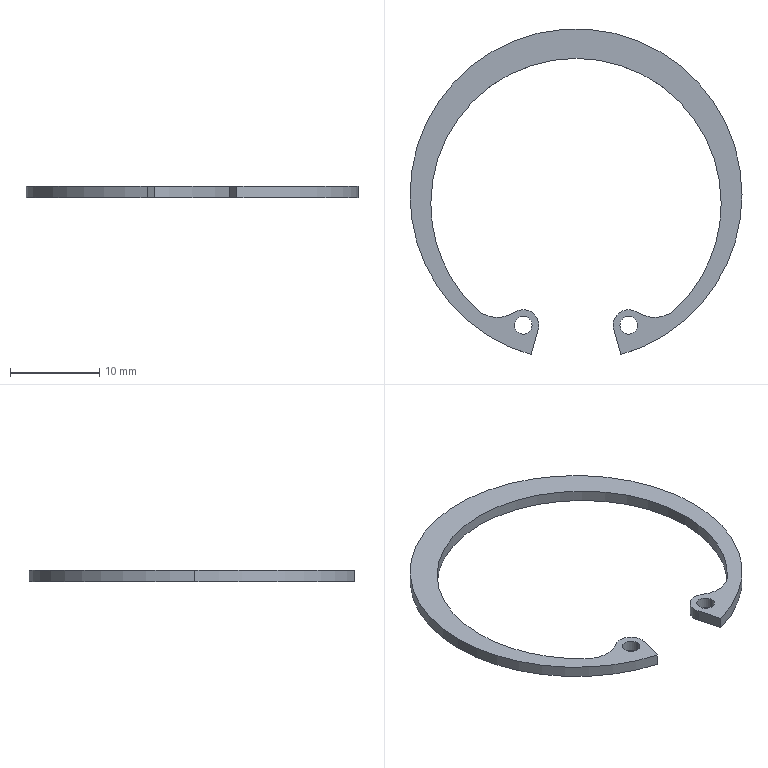Part | STEP file | basic internal retaining ring_wti.25698_Truarc N5000-137 - S1.375 | 1 solid | 19 faces | box 37.109 x 36.419 x 1.27 mm | volume 328.567 mm3 | cylinder 15 | plane 4 | commonest cylinder face diameters 1.981 x4 3.48 x3 32.455 x3 37.109 x3 6.96 x2
STEP:
#1=CARTESIAN_POINT('',(-6.888,-14.575,-1.27));
#2=VERTEX_POINT('',#1);
#3=CARTESIAN_POINT('',(-4.907,-14.575,-1.27));
#4=VERTEX_POINT('',#3);
#5=CARTESIAN_POINT('',(-5.898,-14.575,-1.27));
#6=DIRECTION('',(0.,0.,1.));
#7=DIRECTION('',(1.,0.,0.));
#8=AXIS2_PLACEMENT_3D('',#5,#6,#7);
#9=CIRCLE('',#8,0.9906);
#10=EDGE_CURVE('',#2,#4,#9,.T.);
#11=ORIENTED_EDGE('',*,*,#10,.F.);
#12=CARTESIAN_POINT('',(-6.888,-14.575,0.));
#13=VERTEX_POINT('',#12);
#14=CARTESIAN_POINT('',(-6.888,-14.575,-1.27));
#15=DIRECTION('',(0.,0.,1.));
#16=VECTOR('',#15,1000.);
#17=LINE('',#14,#16);
#18=EDGE_CURVE('',#2,#13,#17,.T.);
#19=ORIENTED_EDGE('',*,*,#18,.T.);
#20=CARTESIAN_POINT('',(-4.907,-14.575,0.));
#21=VERTEX_POINT('',#20);
#22=CARTESIAN_POINT('',(-5.898,-14.575,0.));
#23=DIRECTION('',(0.,0.,1.));
#24=DIRECTION('',(1.,0.,0.));
#25=AXIS2_PLACEMENT_3D('',#22,#23,#24);
#26=CIRCLE('',#25,0.9906);
#27=EDGE_CURVE('',#13,#21,#26,.T.);
#28=ORIENTED_EDGE('',*,*,#27,.T.);
#29=CARTESIAN_POINT('',(-4.907,-14.575,-1.27));
#30=DIRECTION('',(0.,0.,1.));
#31=VECTOR('',#30,1000.);
#32=LINE('',#29,#31);
#33=EDGE_CURVE('',#4,#21,#32,.T.);
#34=ORIENTED_EDGE('',*,*,#33,.F.);
#35=EDGE_LOOP('',(#11,#19,#28,#34));
#36=FACE_OUTER_BOUND('',#35,.T.);
#37=CARTESIAN_POINT('',(-5.898,-14.575,-1.27));
#38=DIRECTION('',(0.,0.,1.));
#39=DIRECTION('',(1.,0.,0.));
#40=AXIS2_PLACEMENT_3D('',#37,#38,#39);
#41=CYLINDRICAL_SURFACE('',#40,0.9906);
#42=ADVANCED_FACE('',(#36),#41,.F.);
#43=CARTESIAN_POINT('',(4.907,-14.575,-1.27));
#44=VERTEX_POINT('',#43);
#45=CARTESIAN_POINT('',(6.888,-14.575,-1.27));
#46=VERTEX_POINT('',#45);
#47=CARTESIAN_POINT('',(5.898,-14.575,-1.27));
#48=DIRECTION('',(0.,0.,1.));
#49=DIRECTION('',(1.,0.,0.));
#50=AXIS2_PLACEMENT_3D('',#47,#48,#49);
#51=CIRCLE('',#50,0.9906);
#52=EDGE_CURVE('',#44,#46,#51,.T.);
#53=ORIENTED_EDGE('',*,*,#52,.F.);
#54=CARTESIAN_POINT('',(4.907,-14.575,0.));
#55=VERTEX_POINT('',#54);
#56=CARTESIAN_POINT('',(4.907,-14.575,-1.27));
#57=DIRECTION('',(0.,0.,1.));
#58=VECTOR('',#57,1000.);
#59=LINE('',#56,#58);
#60=EDGE_CURVE('',#44,#55,#59,.T.);
#61=ORIENTED_EDGE('',*,*,#60,.T.);
#62=CARTESIAN_POINT('',(6.888,-14.575,0.));
#63=VERTEX_POINT('',#62);
#64=CARTESIAN_POINT('',(5.898,-14.575,0.));
#65=DIRECTION('',(0.,0.,1.));
#66=DIRECTION('',(1.,0.,0.));
#67=AXIS2_PLACEMENT_3D('',#64,#65,#66);
#68=CIRCLE('',#67,0.9906);
#69=EDGE_CURVE('',#55,#63,#68,.T.);
#70=ORIENTED_EDGE('',*,*,#69,.T.);
#71=CARTESIAN_POINT('',(6.888,-14.575,-1.27));
#72=DIRECTION('',(0.,0.,1.));
#73=VECTOR('',#72,1000.);
#74=LINE('',#71,#73);
#75=EDGE_CURVE('',#46,#63,#74,.T.);
#76=ORIENTED_EDGE('',*,*,#75,.F.);
#77=EDGE_LOOP('',(#53,#61,#70,#76));
#78=FACE_OUTER_BOUND('',#77,.T.);
#79=CARTESIAN_POINT('',(5.898,-14.575,-1.27));
#80=DIRECTION('',(0.,0.,1.));
#81=DIRECTION('',(1.,0.,0.));
#82=AXIS2_PLACEMENT_3D('',#79,#80,#81);
#83=CYLINDRICAL_SURFACE('',#82,0.9906);
#84=ADVANCED_FACE('',(#78),#83,.F.);
#85=CARTESIAN_POINT('',(-4.223,-15.045,-1.27));
#86=VERTEX_POINT('',#85);
#87=CARTESIAN_POINT('',(-4.158,-14.575,-1.27));
#88=VERTEX_POINT('',#87);
#89=CARTESIAN_POINT('',(-5.898,-14.575,-1.27));
#90=DIRECTION('',(0.,0.,1.));
#91=DIRECTION('',(1.,0.,0.));
#92=AXIS2_PLACEMENT_3D('',#89,#90,#91);
#93=CIRCLE('',#92,1.74);
#94=EDGE_CURVE('',#86,#88,#93,.T.);
#95=ORIENTED_EDGE('',*,*,#94,.T.);
#96=CARTESIAN_POINT('',(-4.158,-14.575,0.));
#97=VERTEX_POINT('',#96);
#98=CARTESIAN_POINT('',(-4.158,-14.575,-1.27));
#99=DIRECTION('',(0.,0.,1.));
#100=VECTOR('',#99,1000.);
#101=LINE('',#98,#100);
#102=EDGE_CURVE('',#88,#97,#101,.T.);
#103=ORIENTED_EDGE('',*,*,#102,.T.);
#104=CARTESIAN_POINT('',(-4.223,-15.045,0.));
#105=VERTEX_POINT('',#104);
#106=CARTESIAN_POINT('',(-5.898,-14.575,0.));
#107=DIRECTION('',(0.,0.,1.));
#108=DIRECTION('',(1.,0.,0.));
#109=AXIS2_PLACEMENT_3D('',#106,#107,#108);
#110=CIRCLE('',#109,1.74);
#111=EDGE_CURVE('',#105,#97,#110,.T.);
#112=ORIENTED_EDGE('',*,*,#111,.F.);
#113=CARTESIAN_POINT('',(-4.223,-15.045,-1.27));
#114=DIRECTION('',(0.,0.,1.));
#115=VECTOR('',#114,1000.);
#116=LINE('',#113,#115);
#117=EDGE_CURVE('',#86,#105,#116,.T.);
#118=ORIENTED_EDGE('',*,*,#117,.F.);
#119=EDGE_LOOP('',(#95,#103,#112,#118));
#120=FACE_OUTER_BOUND('',#119,.T.);
#121=CARTESIAN_POINT('',(-5.898,-14.575,-1.27));
#122=DIRECTION('',(0.,0.,1.));
#123=DIRECTION('',(1.,0.,0.));
#124=AXIS2_PLACEMENT_3D('',#121,#122,#123);
#125=CYLINDRICAL_SURFACE('',#124,1.74);
#126=ADVANCED_FACE('',(#120),#125,.T.);
#127=CARTESIAN_POINT('',(-11.172,-12.744,-1.27));
#128=VERTEX_POINT('',#127);
#129=CARTESIAN_POINT('',(-16.227,-0.9747,-1.27));
#130=VERTEX_POINT('',#129);
#131=CARTESIAN_POINT('',(0.,-0.9747,-1.27));
#132=DIRECTION('',(0.,0.,-1.));
#133=DIRECTION('',(1.,0.,0.));
#134=AXIS2_PLACEMENT_3D('',#131,#132,#133);
#135=CIRCLE('',#134,16.227);
#136=EDGE_CURVE('',#128,#130,#135,.T.);
#137=ORIENTED_EDGE('',*,*,#136,.T.);
#138=CARTESIAN_POINT('',(-16.227,-0.9747,0.));
#139=VERTEX_POINT('',#138);
#140=CARTESIAN_POINT('',(-16.227,-0.9747,-1.27));
#141=DIRECTION('',(0.,0.,1.));
#142=VECTOR('',#141,1000.);
#143=LINE('',#140,#142);
#144=EDGE_CURVE('',#130,#139,#143,.T.);
#145=ORIENTED_EDGE('',*,*,#144,.T.);
#146=CARTESIAN_POINT('',(-11.172,-12.744,0.));
#147=VERTEX_POINT('',#146);
#148=CARTESIAN_POINT('',(0.,-0.9747,0.));
#149=DIRECTION('',(0.,0.,-1.));
#150=DIRECTION('',(1.,0.,0.));
#151=AXIS2_PLACEMENT_3D('',#148,#149,#150);
#152=CIRCLE('',#151,16.227);
#153=EDGE_CURVE('',#147,#139,#152,.T.);
#154=ORIENTED_EDGE('',*,*,#153,.F.);
#155=CARTESIAN_POINT('',(-11.172,-12.744,-1.27));
#156=DIRECTION('',(0.,0.,1.));
#157=VECTOR('',#156,1000.);
#158=LINE('',#155,#157);
#159=EDGE_CURVE('',#128,#147,#158,.T.);
#160=ORIENTED_EDGE('',*,*,#159,.F.);
#161=EDGE_LOOP('',(#137,#145,#154,#160));
#162=FACE_OUTER_BOUND('',#161,.T.);
#163=CARTESIAN_POINT('',(0.,-0.9747,-1.27));
#164=DIRECTION('',(0.,0.,1.));
#165=DIRECTION('',(1.,0.,0.));
#166=AXIS2_PLACEMENT_3D('',#163,#164,#165);
#167=CYLINDRICAL_SURFACE('',#166,16.227);
#168=ADVANCED_FACE('',(#162),#167,.F.);
#169=ORIENTED_EDGE('',*,*,#144,.F.);
#170=CARTESIAN_POINT('',(16.227,-0.9747,-1.27));
#171=VERTEX_POINT('',#170);
#172=CARTESIAN_POINT('',(0.,-0.9747,-1.27));
#173=DIRECTION('',(0.,0.,-1.));
#174=DIRECTION('',(1.,0.,0.));
#175=AXIS2_PLACEMENT_3D('',#172,#173,#174);
#176=CIRCLE('',#175,16.227);
#177=EDGE_CURVE('',#130,#171,#176,.T.);
#178=ORIENTED_EDGE('',*,*,#177,.T.);
#179=CARTESIAN_POINT('',(16.227,-0.9747,0.));
#180=VERTEX_POINT('',#179);
#181=CARTESIAN_POINT('',(16.227,-0.9747,-1.27));
#182=DIRECTION('',(0.,0.,1.));
#183=VECTOR('',#182,1000.);
#184=LINE('',#181,#183);
#185=EDGE_CURVE('',#171,#180,#184,.T.);
#186=ORIENTED_EDGE('',*,*,#185,.T.);
#187=CARTESIAN_POINT('',(0.,-0.9747,0.));
#188=DIRECTION('',(0.,0.,-1.));
#189=DIRECTION('',(1.,0.,0.));
#190=AXIS2_PLACEMENT_3D('',#187,#188,#189);
#191=CIRCLE('',#190,16.227);
#192=EDGE_CURVE('',#139,#180,#191,.T.);
#193=ORIENTED_EDGE('',*,*,#192,.F.);
#194=EDGE_LOOP('',(#169,#178,#186,#193));
#195=FACE_OUTER_BOUND('',#194,.T.);
#196=CARTESIAN_POINT('',(0.,-0.9747,-1.27));
#197=DIRECTION('',(0.,0.,1.));
#198=DIRECTION('',(1.,0.,0.));
#199=AXIS2_PLACEMENT_3D('',#196,#197,#198);
#200=CYLINDRICAL_SURFACE('',#199,16.227);
#201=ADVANCED_FACE('',(#195),#200,.F.);
#202=CARTESIAN_POINT('',(18.555,0.,-1.27));
#203=VERTEX_POINT('',#202);
#204=CARTESIAN_POINT('',(-18.555,0.,-1.27));
#205=VERTEX_POINT('',#204);
#206=CARTESIAN_POINT('',(0.,0.,-1.27));
#207=DIRECTION('',(0.,0.,1.));
#208=DIRECTION('',(1.,0.,0.));
#209=AXIS2_PLACEMENT_3D('',#206,#207,#208);
#210=CIRCLE('',#209,18.555);
#211=EDGE_CURVE('',#203,#205,#210,.T.);
#212=ORIENTED_EDGE('',*,*,#211,.T.);
#213=CARTESIAN_POINT('',(-18.555,0.,0.));
#214=VERTEX_POINT('',#213);
#215=CARTESIAN_POINT('',(-18.555,0.,-1.27));
#216=DIRECTION('',(0.,0.,1.));
#217=VECTOR('',#216,1000.);
#218=LINE('',#215,#217);
#219=EDGE_CURVE('',#205,#214,#218,.T.);
#220=ORIENTED_EDGE('',*,*,#219,.T.);
#221=CARTESIAN_POINT('',(18.555,0.,0.));
#222=VERTEX_POINT('',#221);
#223=CARTESIAN_POINT('',(0.,0.,0.));
#224=DIRECTION('',(0.,0.,1.));
#225=DIRECTION('',(1.,0.,0.));
#226=AXIS2_PLACEMENT_3D('',#223,#224,#225);
#227=CIRCLE('',#226,18.555);
#228=EDGE_CURVE('',#222,#214,#227,.T.);
#229=ORIENTED_EDGE('',*,*,#228,.F.);
#230=CARTESIAN_POINT('',(18.555,0.,-1.27));
#231=DIRECTION('',(0.,0.,1.));
#232=VECTOR('',#231,1000.);
#233=LINE('',#230,#232);
#234=EDGE_CURVE('',#203,#222,#233,.T.);
#235=ORIENTED_EDGE('',*,*,#234,.F.);
#236=EDGE_LOOP('',(#212,#220,#229,#235));
#237=FACE_OUTER_BOUND('',#236,.T.);
#238=CARTESIAN_POINT('',(0.,0.,-1.27));
#239=DIRECTION('',(0.,0.,1.));
#240=DIRECTION('',(1.,0.,0.));
#241=AXIS2_PLACEMENT_3D('',#238,#239,#240);
#242=CYLINDRICAL_SURFACE('',#241,18.555);
#243=ADVANCED_FACE('',(#237),#242,.T.);
#244=CARTESIAN_POINT('',(5.014,-17.864,-1.27));
#245=VERTEX_POINT('',#244);
#246=CARTESIAN_POINT('',(0.,0.,-1.27));
#247=DIRECTION('',(0.,0.,1.));
#248=DIRECTION('',(1.,0.,0.));
#249=AXIS2_PLACEMENT_3D('',#246,#247,#248);
#250=CIRCLE('',#249,18.555);
#251=EDGE_CURVE('',#245,#203,#250,.T.);
#252=ORIENTED_EDGE('',*,*,#251,.T.);
#253=ORIENTED_EDGE('',*,*,#234,.T.);
#254=CARTESIAN_POINT('',(5.014,-17.864,0.));
#255=VERTEX_POINT('',#254);
#256=CARTESIAN_POINT('',(0.,0.,0.));
#257=DIRECTION('',(0.,0.,1.));
#258=DIRECTION('',(1.,0.,0.));
#259=AXIS2_PLACEMENT_3D('',#256,#257,#258);
#260=CIRCLE('',#259,18.555);
#261=EDGE_CURVE('',#255,#222,#260,.T.);
#262=ORIENTED_EDGE('',*,*,#261,.F.);
#263=CARTESIAN_POINT('',(5.014,-17.864,-1.27));
#264=DIRECTION('',(0.,0.,1.));
#265=VECTOR('',#264,1000.);
#266=LINE('',#263,#265);
#267=EDGE_CURVE('',#245,#255,#266,.T.);
#268=ORIENTED_EDGE('',*,*,#267,.F.);
#269=EDGE_LOOP('',(#252,#253,#262,#268));
#270=FACE_OUTER_BOUND('',#269,.T.);
#271=CARTESIAN_POINT('',(0.,0.,-1.27));
#272=DIRECTION('',(0.,0.,1.));
#273=DIRECTION('',(1.,0.,0.));
#274=AXIS2_PLACEMENT_3D('',#271,#272,#273);
#275=CYLINDRICAL_SURFACE('',#274,18.555);
#276=ADVANCED_FACE('',(#270),#275,.T.);
#277=ORIENTED_EDGE('',*,*,#219,.F.);
#278=CARTESIAN_POINT('',(-5.014,-17.864,-1.27));
#279=VERTEX_POINT('',#278);
#280=CARTESIAN_POINT('',(0.,0.,-1.27));
#281=DIRECTION('',(0.,0.,1.));
#282=DIRECTION('',(1.,0.,0.));
#283=AXIS2_PLACEMENT_3D('',#280,#281,#282);
#284=CIRCLE('',#283,18.555);
#285=EDGE_CURVE('',#205,#279,#284,.T.);
#286=ORIENTED_EDGE('',*,*,#285,.T.);
#287=CARTESIAN_POINT('',(-5.014,-17.864,0.));
#288=VERTEX_POINT('',#287);
#289=CARTESIAN_POINT('',(-5.014,-17.864,-1.27));
#290=DIRECTION('',(0.,0.,1.));
#291=VECTOR('',#290,1000.);
#292=LINE('',#289,#291);
#293=EDGE_CURVE('',#279,#288,#292,.T.);
#294=ORIENTED_EDGE('',*,*,#293,.T.);
#295=CARTESIAN_POINT('',(0.,0.,0.));
#296=DIRECTION('',(0.,0.,1.));
#297=DIRECTION('',(1.,0.,0.));
#298=AXIS2_PLACEMENT_3D('',#295,#296,#297);
#299=CIRCLE('',#298,18.555);
#300=EDGE_CURVE('',#214,#288,#299,.T.);
#301=ORIENTED_EDGE('',*,*,#300,.F.);
#302=EDGE_LOOP('',(#277,#286,#294,#301));
#303=FACE_OUTER_BOUND('',#302,.T.);
#304=CARTESIAN_POINT('',(0.,0.,-1.27));
#305=DIRECTION('',(0.,0.,1.));
#306=DIRECTION('',(1.,0.,0.));
#307=AXIS2_PLACEMENT_3D('',#304,#305,#306);
#308=CYLINDRICAL_SURFACE('',#307,18.555);
#309=ADVANCED_FACE('',(#303),#308,.T.);
#310=CARTESIAN_POINT('',(4.223,-15.045,0.));
#311=VERTEX_POINT('',#310);
#312=CARTESIAN_POINT('',(5.014,-17.864,0.));
#313=DIRECTION('',(0.2702,-0.9628,0.));
#314=VECTOR('',#313,1000.);
#315=LINE('',#312,#314);
#316=EDGE_CURVE('',#311,#255,#315,.T.);
#317=ORIENTED_EDGE('',*,*,#316,.F.);
#318=CARTESIAN_POINT('',(4.223,-15.045,-1.27));
#319=VERTEX_POINT('',#318);
#320=CARTESIAN_POINT('',(4.223,-15.045,-1.27));
#321=DIRECTION('',(0.,0.,1.));
#322=VECTOR('',#321,1000.);
#323=LINE('',#320,#322);
#324=EDGE_CURVE('',#319,#311,#323,.T.);
#325=ORIENTED_EDGE('',*,*,#324,.F.);
#326=CARTESIAN_POINT('',(5.014,-17.864,-1.27));
#327=DIRECTION('',(0.2702,-0.9628,0.));
#328=VECTOR('',#327,1000.);
#329=LINE('',#326,#328);
#330=EDGE_CURVE('',#319,#245,#329,.T.);
#331=ORIENTED_EDGE('',*,*,#330,.T.);
#332=ORIENTED_EDGE('',*,*,#267,.T.);
#333=EDGE_LOOP('',(#317,#325,#331,#332));
#334=FACE_OUTER_BOUND('',#333,.T.);
#335=CARTESIAN_POINT('',(5.014,-17.864,-1.27));
#336=DIRECTION('',(-0.9628,-0.2702,0.));
#337=DIRECTION('',(0.2702,-0.9628,0.));
#338=AXIS2_PLACEMENT_3D('',#335,#336,#337);
#339=PLANE('',#338);
#340=ADVANCED_FACE('',(#334),#339,.T.);
#341=CARTESIAN_POINT('',(6.857,-13.123,0.));
#342=VERTEX_POINT('',#341);
#343=CARTESIAN_POINT('',(5.898,-14.575,0.));
#344=DIRECTION('',(0.,0.,1.));
#345=DIRECTION('',(1.,0.,0.));
#346=AXIS2_PLACEMENT_3D('',#343,#344,#345);
#347=CIRCLE('',#346,1.74);
#348=EDGE_CURVE('',#342,#311,#347,.T.);
#349=ORIENTED_EDGE('',*,*,#348,.F.);
#350=CARTESIAN_POINT('',(6.857,-13.123,-1.27));
#351=VERTEX_POINT('',#350);
#352=CARTESIAN_POINT('',(6.857,-13.123,-1.27));
#353=DIRECTION('',(0.,0.,1.));
#354=VECTOR('',#353,1000.);
#355=LINE('',#352,#354);
#356=EDGE_CURVE('',#351,#342,#355,.T.);
#357=ORIENTED_EDGE('',*,*,#356,.F.);
#358=CARTESIAN_POINT('',(5.898,-14.575,-1.27));
#359=DIRECTION('',(0.,0.,1.));
#360=DIRECTION('',(1.,0.,0.));
#361=AXIS2_PLACEMENT_3D('',#358,#359,#360);
#362=CIRCLE('',#361,1.74);
#363=EDGE_CURVE('',#351,#319,#362,.T.);
#364=ORIENTED_EDGE('',*,*,#363,.T.);
#365=ORIENTED_EDGE('',*,*,#324,.T.);
#366=EDGE_LOOP('',(#349,#357,#364,#365));
#367=FACE_OUTER_BOUND('',#366,.T.);
#368=CARTESIAN_POINT('',(5.898,-14.575,-1.27));
#369=DIRECTION('',(0.,0.,1.));
#370=DIRECTION('',(1.,0.,0.));
#371=AXIS2_PLACEMENT_3D('',#368,#369,#370);
#372=CYLINDRICAL_SURFACE('',#371,1.74);
#373=ADVANCED_FACE('',(#367),#372,.T.);
#374=CARTESIAN_POINT('',(11.172,-12.744,0.));
#375=VERTEX_POINT('',#374);
#376=CARTESIAN_POINT('',(8.776,-10.22,0.));
#377=DIRECTION('',(0.,0.,-1.));
#378=DIRECTION('',(1.,0.,0.));
#379=AXIS2_PLACEMENT_3D('',#376,#377,#378);
#380=CIRCLE('',#379,3.48);
#381=EDGE_CURVE('',#375,#342,#380,.T.);
#382=ORIENTED_EDGE('',*,*,#381,.F.);
#383=CARTESIAN_POINT('',(11.172,-12.744,-1.27));
#384=VERTEX_POINT('',#383);
#385=CARTESIAN_POINT('',(11.172,-12.744,-1.27));
#386=DIRECTION('',(0.,0.,1.));
#387=VECTOR('',#386,1000.);
#388=LINE('',#385,#387);
#389=EDGE_CURVE('',#384,#375,#388,.T.);
#390=ORIENTED_EDGE('',*,*,#389,.F.);
#391=CARTESIAN_POINT('',(8.776,-10.22,-1.27));
#392=DIRECTION('',(0.,0.,-1.));
#393=DIRECTION('',(1.,0.,0.));
#394=AXIS2_PLACEMENT_3D('',#391,#392,#393);
#395=CIRCLE('',#394,3.48);
#396=EDGE_CURVE('',#384,#351,#395,.T.);
#397=ORIENTED_EDGE('',*,*,#396,.T.);
#398=ORIENTED_EDGE('',*,*,#356,.T.);
#399=EDGE_LOOP('',(#382,#390,#397,#398));
#400=FACE_OUTER_BOUND('',#399,.T.);
#401=CARTESIAN_POINT('',(8.776,-10.22,-1.27));
#402=DIRECTION('',(0.,0.,1.));
#403=DIRECTION('',(1.,0.,0.));
#404=AXIS2_PLACEMENT_3D('',#401,#402,#403);
#405=CYLINDRICAL_SURFACE('',#404,3.48);
#406=ADVANCED_FACE('',(#400),#405,.F.);
#407=ORIENTED_EDGE('',*,*,#185,.F.);
#408=CARTESIAN_POINT('',(0.,-0.9747,-1.27));
#409=DIRECTION('',(0.,0.,-1.));
#410=DIRECTION('',(1.,0.,0.));
#411=AXIS2_PLACEMENT_3D('',#408,#409,#410);
#412=CIRCLE('',#411,16.227);
#413=EDGE_CURVE('',#171,#384,#412,.T.);
#414=ORIENTED_EDGE('',*,*,#413,.T.);
#415=ORIENTED_EDGE('',*,*,#389,.T.);
#416=CARTESIAN_POINT('',(0.,-0.9747,0.));
#417=DIRECTION('',(0.,0.,-1.));
#418=DIRECTION('',(1.,0.,0.));
#419=AXIS2_PLACEMENT_3D('',#416,#417,#418);
#420=CIRCLE('',#419,16.227);
#421=EDGE_CURVE('',#180,#375,#420,.T.);
#422=ORIENTED_EDGE('',*,*,#421,.F.);
#423=EDGE_LOOP('',(#407,#414,#415,#422));
#424=FACE_OUTER_BOUND('',#423,.T.);
#425=CARTESIAN_POINT('',(0.,-0.9747,-1.27));
#426=DIRECTION('',(0.,0.,1.));
#427=DIRECTION('',(1.,0.,0.));
#428=AXIS2_PLACEMENT_3D('',#425,#426,#427);
#429=CYLINDRICAL_SURFACE('',#428,16.227);
#430=ADVANCED_FACE('',(#424),#429,.F.);
#431=CARTESIAN_POINT('',(-6.857,-13.123,0.));
#432=VERTEX_POINT('',#431);
#433=CARTESIAN_POINT('',(-8.776,-10.22,0.));
#434=DIRECTION('',(0.,0.,-1.));
#435=DIRECTION('',(1.,0.,0.));
#436=AXIS2_PLACEMENT_3D('',#433,#434,#435);
#437=CIRCLE('',#436,3.48);
#438=EDGE_CURVE('',#432,#147,#437,.T.);
#439=ORIENTED_EDGE('',*,*,#438,.F.);
#440=CARTESIAN_POINT('',(-6.857,-13.123,-1.27));
#441=VERTEX_POINT('',#440);
#442=CARTESIAN_POINT('',(-6.857,-13.123,-1.27));
#443=DIRECTION('',(0.,0.,1.));
#444=VECTOR('',#443,1000.);
#445=LINE('',#442,#444);
#446=EDGE_CURVE('',#441,#432,#445,.T.);
#447=ORIENTED_EDGE('',*,*,#446,.F.);
#448=CARTESIAN_POINT('',(-8.776,-10.22,-1.27));
#449=DIRECTION('',(0.,0.,-1.));
#450=DIRECTION('',(1.,0.,0.));
#451=AXIS2_PLACEMENT_3D('',#448,#449,#450);
#452=CIRCLE('',#451,3.48);
#453=EDGE_CURVE('',#441,#128,#452,.T.);
#454=ORIENTED_EDGE('',*,*,#453,.T.);
#455=ORIENTED_EDGE('',*,*,#159,.T.);
#456=EDGE_LOOP('',(#439,#447,#454,#455));
#457=FACE_OUTER_BOUND('',#456,.T.);
#458=CARTESIAN_POINT('',(-8.776,-10.22,-1.27));
#459=DIRECTION('',(0.,0.,1.));
#460=DIRECTION('',(1.,0.,0.));
#461=AXIS2_PLACEMENT_3D('',#458,#459,#460);
#462=CYLINDRICAL_SURFACE('',#461,3.48);
#463=ADVANCED_FACE('',(#457),#462,.F.);
#464=ORIENTED_EDGE('',*,*,#102,.F.);
#465=CARTESIAN_POINT('',(-5.898,-14.575,-1.27));
#466=DIRECTION('',(0.,0.,1.));
#467=DIRECTION('',(1.,0.,0.));
#468=AXIS2_PLACEMENT_3D('',#465,#466,#467);
#469=CIRCLE('',#468,1.74);
#470=EDGE_CURVE('',#88,#441,#469,.T.);
#471=ORIENTED_EDGE('',*,*,#470,.T.);
#472=ORIENTED_EDGE('',*,*,#446,.T.);
#473=CARTESIAN_POINT('',(-5.898,-14.575,0.));
#474=DIRECTION('',(0.,0.,1.));
#475=DIRECTION('',(1.,0.,0.));
#476=AXIS2_PLACEMENT_3D('',#473,#474,#475);
#477=CIRCLE('',#476,1.74);
#478=EDGE_CURVE('',#97,#432,#477,.T.);
#479=ORIENTED_EDGE('',*,*,#478,.F.);
#480=EDGE_LOOP('',(#464,#471,#472,#479));
#481=FACE_OUTER_BOUND('',#480,.T.);
#482=CARTESIAN_POINT('',(-5.898,-14.575,-1.27));
#483=DIRECTION('',(0.,0.,1.));
#484=DIRECTION('',(1.,0.,0.));
#485=AXIS2_PLACEMENT_3D('',#482,#483,#484);
#486=CYLINDRICAL_SURFACE('',#485,1.74);
#487=ADVANCED_FACE('',(#481),#486,.T.);
#488=CARTESIAN_POINT('',(-5.014,-17.864,0.));
#489=DIRECTION('',(0.2702,0.9628,0.));
#490=VECTOR('',#489,1000.);
#491=LINE('',#488,#490);
#492=EDGE_CURVE('',#288,#105,#491,.T.);
#493=ORIENTED_EDGE('',*,*,#492,.F.);
#494=ORIENTED_EDGE('',*,*,#293,.F.);
#495=CARTESIAN_POINT('',(-5.014,-17.864,-1.27));
#496=DIRECTION('',(0.2702,0.9628,0.));
#497=VECTOR('',#496,1000.);
#498=LINE('',#495,#497);
#499=EDGE_CURVE('',#279,#86,#498,.T.);
#500=ORIENTED_EDGE('',*,*,#499,.T.);
#501=ORIENTED_EDGE('',*,*,#117,.T.);
#502=EDGE_LOOP('',(#493,#494,#500,#501));
#503=FACE_OUTER_BOUND('',#502,.T.);
#504=CARTESIAN_POINT('',(-5.014,-17.864,-1.27));
#505=DIRECTION('',(0.9628,-0.2702,0.));
#506=DIRECTION('',(0.2702,0.9628,0.));
#507=AXIS2_PLACEMENT_3D('',#504,#505,#506);
#508=PLANE('',#507);
#509=ADVANCED_FACE('',(#503),#508,.T.);
#510=CARTESIAN_POINT('',(-5.898,-14.575,-1.27));
#511=DIRECTION('',(0.,0.,1.));
#512=DIRECTION('',(1.,0.,0.));
#513=AXIS2_PLACEMENT_3D('',#510,#511,#512);
#514=CIRCLE('',#513,0.9906);
#515=EDGE_CURVE('',#4,#2,#514,.T.);
#516=ORIENTED_EDGE('',*,*,#515,.T.);
#517=ORIENTED_EDGE('',*,*,#10,.T.);
#518=EDGE_LOOP('',(#516,#517));
#519=FACE_BOUND('',#518,.T.);
#520=CARTESIAN_POINT('',(5.898,-14.575,-1.27));
#521=DIRECTION('',(0.,0.,1.));
#522=DIRECTION('',(1.,0.,0.));
#523=AXIS2_PLACEMENT_3D('',#520,#521,#522);
#524=CIRCLE('',#523,0.9906);
#525=EDGE_CURVE('',#46,#44,#524,.T.);
#526=ORIENTED_EDGE('',*,*,#525,.T.);
#527=ORIENTED_EDGE('',*,*,#52,.T.);
#528=EDGE_LOOP('',(#526,#527));
#529=FACE_BOUND('',#528,.T.);
#530=ORIENTED_EDGE('',*,*,#251,.F.);
#531=ORIENTED_EDGE('',*,*,#330,.F.);
#532=ORIENTED_EDGE('',*,*,#363,.F.);
#533=ORIENTED_EDGE('',*,*,#396,.F.);
#534=ORIENTED_EDGE('',*,*,#413,.F.);
#535=ORIENTED_EDGE('',*,*,#177,.F.);
#536=ORIENTED_EDGE('',*,*,#136,.F.);
#537=ORIENTED_EDGE('',*,*,#453,.F.);
#538=ORIENTED_EDGE('',*,*,#470,.F.);
#539=ORIENTED_EDGE('',*,*,#94,.F.);
#540=ORIENTED_EDGE('',*,*,#499,.F.);
#541=ORIENTED_EDGE('',*,*,#285,.F.);
#542=ORIENTED_EDGE('',*,*,#211,.F.);
#543=EDGE_LOOP('',(#530,#531,#532,#533,#534,#535,#536,#537,#538,#539,#540,#541,#542));
#544=FACE_OUTER_BOUND('',#543,.T.);
#545=CARTESIAN_POINT('',(0.,0.,-1.27));
#546=DIRECTION('',(0.,0.,1.));
#547=DIRECTION('',(1.,0.,0.));
#548=AXIS2_PLACEMENT_3D('',#545,#546,#547);
#549=PLANE('',#548);
#550=ADVANCED_FACE('',(#519,#529,#544),#549,.F.);
#551=CARTESIAN_POINT('',(-5.898,-14.575,0.));
#552=DIRECTION('',(0.,0.,1.));
#553=DIRECTION('',(1.,0.,0.));
#554=AXIS2_PLACEMENT_3D('',#551,#552,#553);
#555=CIRCLE('',#554,0.9906);
#556=EDGE_CURVE('',#21,#13,#555,.T.);
#557=ORIENTED_EDGE('',*,*,#556,.F.);
#558=ORIENTED_EDGE('',*,*,#27,.F.);
#559=EDGE_LOOP('',(#557,#558));
#560=FACE_BOUND('',#559,.T.);
#561=CARTESIAN_POINT('',(5.898,-14.575,0.));
#562=DIRECTION('',(0.,0.,1.));
#563=DIRECTION('',(1.,0.,0.));
#564=AXIS2_PLACEMENT_3D('',#561,#562,#563);
#565=CIRCLE('',#564,0.9906);
#566=EDGE_CURVE('',#63,#55,#565,.T.);
#567=ORIENTED_EDGE('',*,*,#566,.F.);
#568=ORIENTED_EDGE('',*,*,#69,.F.);
#569=EDGE_LOOP('',(#567,#568));
#570=FACE_BOUND('',#569,.T.);
#571=ORIENTED_EDGE('',*,*,#261,.T.);
#572=ORIENTED_EDGE('',*,*,#228,.T.);
#573=ORIENTED_EDGE('',*,*,#300,.T.);
#574=ORIENTED_EDGE('',*,*,#492,.T.);
#575=ORIENTED_EDGE('',*,*,#111,.T.);
#576=ORIENTED_EDGE('',*,*,#478,.T.);
#577=ORIENTED_EDGE('',*,*,#438,.T.);
#578=ORIENTED_EDGE('',*,*,#153,.T.);
#579=ORIENTED_EDGE('',*,*,#192,.T.);
#580=ORIENTED_EDGE('',*,*,#421,.T.);
#581=ORIENTED_EDGE('',*,*,#381,.T.);
#582=ORIENTED_EDGE('',*,*,#348,.T.);
#583=ORIENTED_EDGE('',*,*,#316,.T.);
#584=EDGE_LOOP('',(#571,#572,#573,#574,#575,#576,#577,#578,#579,#580,#581,#582,#583));
#585=FACE_OUTER_BOUND('',#584,.T.);
#586=CARTESIAN_POINT('',(0.,0.,0.));
#587=DIRECTION('',(0.,0.,1.));
#588=DIRECTION('',(1.,0.,0.));
#589=AXIS2_PLACEMENT_3D('',#586,#587,#588);
#590=PLANE('',#589);
#591=ADVANCED_FACE('',(#560,#570,#585),#590,.T.);
#592=ORIENTED_EDGE('',*,*,#60,.F.);
#593=ORIENTED_EDGE('',*,*,#525,.F.);
#594=ORIENTED_EDGE('',*,*,#75,.T.);
#595=ORIENTED_EDGE('',*,*,#566,.T.);
#596=EDGE_LOOP('',(#592,#593,#594,#595));
#597=FACE_OUTER_BOUND('',#596,.T.);
#598=CARTESIAN_POINT('',(5.898,-14.575,-1.27));
#599=DIRECTION('',(0.,0.,1.));
#600=DIRECTION('',(1.,0.,0.));
#601=AXIS2_PLACEMENT_3D('',#598,#599,#600);
#602=CYLINDRICAL_SURFACE('',#601,0.9906);
#603=ADVANCED_FACE('',(#597),#602,.F.);
#604=ORIENTED_EDGE('',*,*,#18,.F.);
#605=ORIENTED_EDGE('',*,*,#515,.F.);
#606=ORIENTED_EDGE('',*,*,#33,.T.);
#607=ORIENTED_EDGE('',*,*,#556,.T.);
#608=EDGE_LOOP('',(#604,#605,#606,#607));
#609=FACE_OUTER_BOUND('',#608,.T.);
#610=CARTESIAN_POINT('',(-5.898,-14.575,-1.27));
#611=DIRECTION('',(0.,0.,1.));
#612=DIRECTION('',(1.,0.,0.));
#613=AXIS2_PLACEMENT_3D('',#610,#611,#612);
#614=CYLINDRICAL_SURFACE('',#613,0.9906);
#615=ADVANCED_FACE('',(#609),#614,.F.);
#616=CLOSED_SHELL('',(#42,#84,#126,#168,#201,#243,#276,#309,#340,#373,#406,#430,#463,#487,#509,#550,#591,#603,#615));
#617=MANIFOLD_SOLID_BREP('',#616);
#618=CARTESIAN_POINT('',(0.,0.,0.));
#619=DIRECTION('',(0.,0.,1.));
#620=DIRECTION('',(1.,0.,0.));
#621=AXIS2_PLACEMENT_3D('',#618,#619,#620);
#622=(LENGTH_UNIT()NAMED_UNIT(*)SI_UNIT(.MILLI.,.METRE.));
#623=UNCERTAINTY_MEASURE_WITH_UNIT(LENGTH_MEASURE(0.00001),#622,'','');
#624=(NAMED_UNIT(*)PLANE_ANGLE_UNIT()SI_UNIT($,.RADIAN.));
#625=(NAMED_UNIT(*)SI_UNIT($,.STERADIAN.)SOLID_ANGLE_UNIT());
#626=(GEOMETRIC_REPRESENTATION_CONTEXT(3)GLOBAL_UNCERTAINTY_ASSIGNED_CONTEXT((#623))GLOBAL_UNIT_ASSIGNED_CONTEXT((#622,#624,#625))REPRESENTATION_CONTEXT('',''));
#627=ADVANCED_BREP_SHAPE_REPRESENTATION('',(#617,#621),#626);